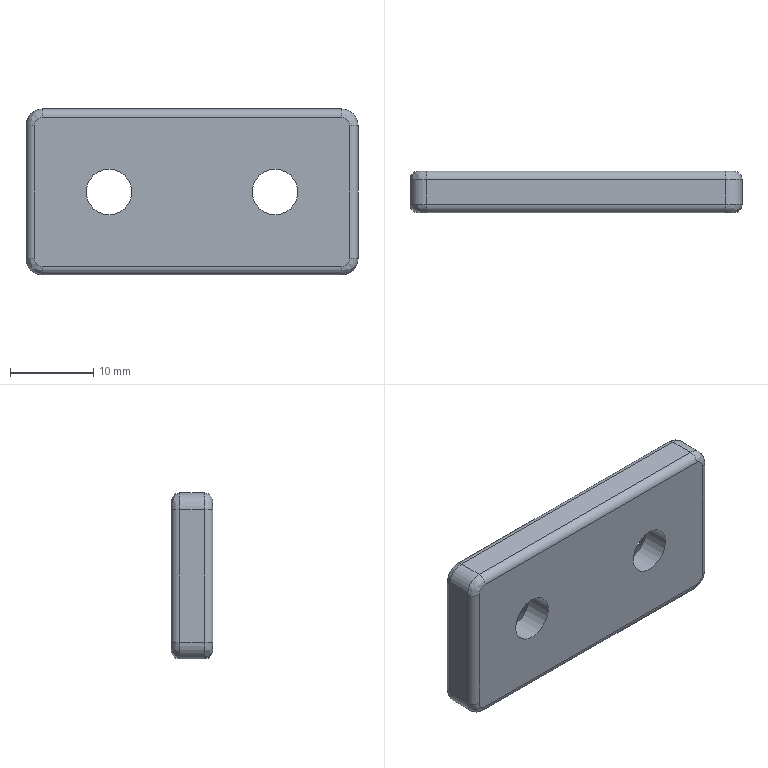Part | STEP file | Door magnet catch | 1 solid | 30 faces | box 40 x 5 x 20 mm | volume 3632 mm3 | cylinder 14 | spline 8 | plane 6 | cone 2 | commonest cylinder face diameters 2 x8 4 x4 5.5 x2